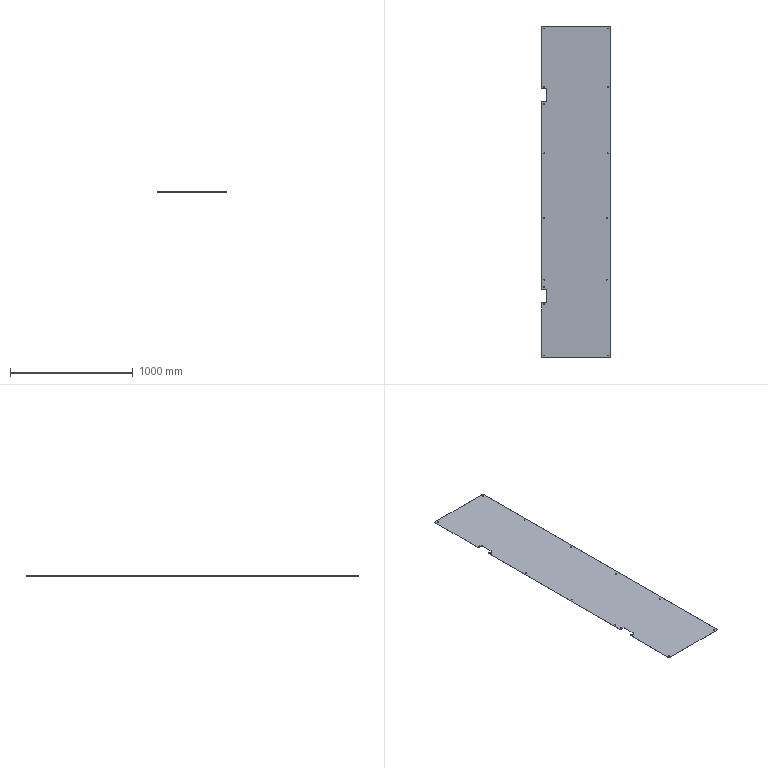Part | SolidWorks | features Cut 1, Fillet 1, FlatPattern 1, HoleWzd 1, SMBaseFlange 1, SheetMetal 1 | 1 solid | 56 faces | box 560 x 2710 x 1.2 mm | volume 1810338 mm3 | cylinder 42 | plane 14 | commonest cylinder face diameters 7 x30 6 x12